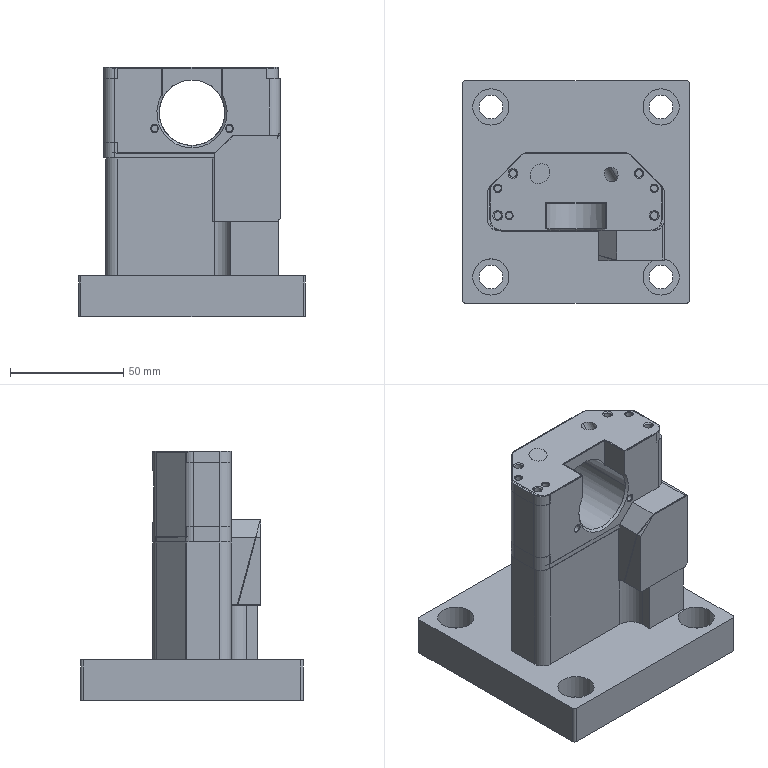NC program | NX | posted with a generic post | part box 100 x 98 x 110 mm
Lines 1874 to 3149 of 3149:
(FLOOR_WALL_2 , TOOL : D8-25-D8-60-3T-FINISH)
N3686 T27 M6
N3688 G54
N3690 G17 G43 G0 G90 X25.696 Y-29.571 B0. C219.917 S4500 H27 M3
N3692 Z33.
N3694 Z3.
N3696 G94 G1 Z0. F800.
N3698 X25.851 Y-29.385
N3700 G3 X25.601 Y-26.568 R2.
N3702 G1 X6.074 Y-10.231
N3704 X5.457 Y-3.296
N3706 X5.618 Y-3.103
N3708 X32.769 Y-25.818
N3710 X36.09 Y-21.849
N3712 X8.939 Y0.866
N3714 X12.259 Y4.835
N3716 X39.41 Y-17.88
N3718 X42.731 Y-13.911
N3720 X15.58 Y8.804
N3722 G3 X12.763 Y8.553 R2.
N3724 G1 X11.996 Y9.195
N3726 Z3.
N3728 G0 Z33.
(PLANAR_MILL_24_COPY , TOOL : D8-25-D8-60-3T-FINISH)
N3730 X12.191 Y-35.298
N3732 Z2.
N3734 Z-25.
N3736 G1 Z-28.
N3738 X6.055 Y-30.164
N3740 X-30.76 Y0.636
N3742 X-36.896 Y5.769
N3744 Z-25.
N3746 G0 Z2.
(FLOOR_WALL_1_COPY_2 , TOOL : D8-25-D8-60-3T-FINISH)
N3748 Z30.2
N3750 X18.538 Y-33.722
N3752 Z-27.
N3754 G1 Z-30.
N3756 X18.694 Y-33.536
N3758 G3 X18.443 Y-30.718 R2.
N3760 G1 X14.105 Y-27.089
N3762 X14.538 Y-26.57
N3764 X-28.719 Y9.62
N3766 X-29.153 Y9.102
N3768 X-33.492 Y12.732
N3770 X-34.28 Y21.599
N3772 X-34.289 Y21.703
N3774 X5.708 Y-11.76
N3776 X4.94 Y-3.134
N3778 X5.098 Y-2.945
N3780 X-31.333 Y27.534
N3782 X-27.247 Y32.419
N3784 X9.185 Y1.939
N3786 X13.271 Y6.824
N3788 X-23.06 Y37.22
N3790 G3 X-25.877 Y36.97 R2.
N3792 G1 X-26.744 Y37.695
N3794 Z-27.
N3796 G0 Z30.2
N3798 X24.693 Y-33.174
N3800 Z-27.
N3802 G1 Z-30.
N3804 X24.161 Y-27.198
N3806 X27.414 Y-29.92
N3808 G2 X27.665 Y-32.737 R2.
N3810 G1 X27.509 Y-32.924
N3812 Z-27.
N3814 G0 Z30.2
(PLANAR_MILL_25 , TOOL : D8-25-D8-60-3T-FINISH)
N3816 X38.714 Y-25.703
N3818 Z30.
N3820 Z-12.
N3822 G1 Z-15.
N3824 X30.745 Y-26.412
N3826 X18.702 Y-27.483
N3828 G2 X15.78 Y-26.566 R4.
N3830 G1 X7.809 Y-19.897
N3832 G2 X6.391 Y-17.184 R4.
N3834 G1 X5.294 Y-4.849
N3836 G2 X6.21 Y-1.928 R4.
N3838 G1 X22.564 Y17.619
N3840 X27.697 Y23.755
N3842 Z-12.
N3844 G0 Z30.
N3846 X38.714 Y-25.703
N3848 Z-12.
N3850 G1 Z-15.
N3852 X30.745 Y-26.412
N3854 X18.702 Y-27.483
N3856 G2 X15.78 Y-26.566 R4.
N3858 G1 X7.809 Y-19.897
N3860 G2 X6.391 Y-17.184 R4.
N3862 G1 X5.294 Y-4.849
N3864 G2 X6.21 Y-1.928 R4.
N3866 G1 X22.564 Y17.619
N3868 X27.697 Y23.755
N3870 Z-12.
N3872 G0 Z30.
N3874 X38.714 Y-25.703
N3876 Z-27.
N3878 G1 Z-30.
N3880 X30.745 Y-26.412
N3882 X18.702 Y-27.483
N3884 G2 X15.78 Y-26.566 R4.
N3886 G1 X7.809 Y-19.897
N3888 G2 X6.391 Y-17.184 R4.
N3890 G1 X5.294 Y-4.849
N3892 G2 X6.21 Y-1.928 R4.
N3894 G1 X22.564 Y17.619
N3896 X27.697 Y23.755
N3898 Z-27.
N3900 G0 Z30.
N3902 X38.714 Y-25.703
N3904 Z-27.
N3906 G1 Z-30.
N3908 X30.745 Y-26.412
N3910 X18.702 Y-27.483
N3912 G2 X15.78 Y-26.566 R4.
N3914 G1 X7.809 Y-19.897
N3916 G2 X6.391 Y-17.184 R4.
N3918 G1 X5.294 Y-4.849
N3920 G2 X6.21 Y-1.928 R4.
N3922 G1 X22.564 Y17.619
N3924 X27.697 Y23.755
N3926 Z-27.
N3928 G0 Z30.
(PLANAR_MILL_25_COPY_2 , TOOL : D8-25-D8-60-3T-FINISH)
N3930 X1.13 Y-8.108
N3932 Z-11.998
N3934 G1 Z-14.998
N3936 X6.264 Y-1.973
N3938 X22.617 Y17.574
N3940 X27.751 Y23.71
N3942 Z-11.998
N3944 G0 Z30.
N3946 X1.13 Y-8.108
N3948 Z-26.996
N3950 G1 Z-29.996
N3952 X6.264 Y-1.973
N3954 X22.617 Y17.574
N3956 X27.751 Y23.71
N3958 Z-26.996
N3960 G0 Z30.
(PLANAR_MILL_25_COPY_1 , TOOL : D8-25-D8-60-3T-FINISH)
N3962 X-37.05 Y-0.649
N3964 Z2.
N3966 Z-26.996
N3968 G1 Z-29.996
N3970 X-31.916 Y5.487
N3972 X-31.261 Y6.27
N3974 G2 X-25.626 Y6.772 R4.
N3976 G1 X11.189 Y-24.029
N3978 G2 X11.69 Y-29.663 R4.
N3980 G1 X11.034 Y-30.447
N3982 X5.901 Y-36.583
N3984 Z-26.996
N3986 G0 Z2.
N3988 X-37.05 Y-0.649
N3990 Z-26.996
N3992 G1 Z-29.996
N3994 X-31.916 Y5.487
N3996 X-31.261 Y6.27
N3998 G2 X-25.626 Y6.772 R4.
N4000 G1 X11.189 Y-24.029
N4002 G2 X11.69 Y-29.663 R4.
N4004 G1 X11.034 Y-30.447
N4006 X5.901 Y-36.583
N4008 Z-26.996
N4010 G0 Z2.
(FLOOR_WALL_1_COPY_3_COPY , TOOL : D8-25-D8-60-3T-FINISH)
N4012 Z30.
N4014 X0.916 Y-11.523
N4016 Z-26.1
N4018 G1 Z-29.1
N4020 X-1.009 Y-13.824
N4022 X-7.425 Y-21.494
N4024 X-11.566 Y-18.03
N4026 X-5.15 Y-10.36
N4028 X-9.29 Y-6.895
N4030 X-15.707 Y-14.565
N4032 X-19.848 Y-11.101
N4034 X-13.431 Y-3.431
N4036 X-11.506 Y-1.13
N4038 Z-26.1
N4040 G0 Z30.
(PLANAR_MILL_35_COPY , TOOL : D8-25-D8-60-3T-FINISH)
N4042 X-36.493 Y24.952
N4044 Z0.
N4046 Z-33.
N4048 G1 Z-35.
N4050 G3 X-33.675 Y25.202 R2.
N4052 G1 X-24.353 Y36.346
N4054 G2 X-11.675 Y37.474 R9.
N4056 G3 X-8.857 Y37.724 R2.
N4058 G1 Z-33.
N4060 G0 Z0.
(FLOOR_WALL_1_COPY_1_1_COPY , TOOL : D8-25-D8-60-3T-FINISH)
N4062 G3P2 X0. Y0. Z0. I0. J74.9748 K-39.9168
N4064 G53.1
N4066 X22.176 Y-36.663 Z55.558 H27
N4068 Z22.558
N4070 G1 Z19.558
N4072 X18.977 Y-39.339
N4074 X-4.808 Y-59.239
N4076 X-8.388 Y-54.96
N4078 X18.763 Y-32.245
N4080 X15.183 Y-27.966
N4082 X-11.968 Y-50.681
N4084 X-15.548 Y-46.402
N4086 X11.603 Y-23.686
N4088 X8.023 Y-19.407
N4090 X-19.128 Y-42.123
N4092 X-22.708 Y-37.844
N4094 X4.443 Y-15.128
N4096 X0.863 Y-10.849
N4098 X-26.288 Y-33.564
N4100 X-28.589 Y-35.489
N4102 Z22.558
N4104 G0 Z55.558
N4106 G69
N4108 M5
(DRILLING_7 , TOOL : 点孔D6-65-90度)
N4110 T04 M6
N4112 G54
N4114 G17 G43 G0 G90 X-2.363 Y-13.734 B0. C219.917 S2500 H4 M3
N4116 Z-27.
N4118 G94 G81 G98 Z-32. F200. R-27.
N4120 X-13.101 Y-4.75
N4122 X-16.573 Y20.71
N4124 G80
N4126 M5
(DRILLING_1_COPY , TOOL : D6-18-D6-50-3T-ROUGH)
N4128 T33 M6
N4130 G54
N4132 G17 G0 G90 X21.776 Y-11.374 B0. C219.917 S1600 M3
N4134 G43 Z3. H33
N4136 G94 G83 G99 Z-22.6 F150. Q5. R3.
N4138 G80
N4140 M5
(SPOT_DRILLING_14 , TOOL : 钻头D3.3-45-73)
N4142 T10 M6
N4144 G54
N4146 G17 G0 G90 X-2.363 Y-13.734 B0. C219.917 S3000 M3
N4148 G43 Z0. H10
N4150 G94 G81 G98 Z-39. F200. R-27.
N4152 X-13.101 Y-4.75
N4154 G80
N4156 M5
(DRILLING_9 , TOOL : D15.3)
N4158 T29 M6
N4160 G54
N4162 G17 G0 G90 X-16.573 Y20.71 B0. C219.917 S1600 M3
N4164 G43 Z-27. H29
N4166 G94 G83 G99 Z-56.797 F150. Q5. R-27.
N4168 G80
N4170 M5
(PLANAR_MILL_37 , TOOL : D8-25-D8-60-3T-ROUGH)
N4172 T26 M6
N4174 G54
N4176 G17 G0 G90 X19.98 Y-10.783 B0. C219.917 S4500 M3
N4178 G43 Z30. H26
N4180 Z2.
N4182 G94 G1 X19.859 Y-11.154 Z1.98 F1000.
N4184 X19.928 Y-11.929 Z1.939
N4186 X20.297 Y-12.613 Z1.898
N4188 X20.817 Y-13.048 Z1.863
N4190 X21.556 Y-13.291 Z1.822
N4192 X22.331 Y-13.222 Z1.781
N4194 X23.016 Y-12.853 Z1.74
N4196 X23.451 Y-12.333 Z1.705
N4198 X23.694 Y-11.594 Z1.664
N4200 X23.625 Y-10.819 Z1.623
N4202 X23.255 Y-10.134 Z1.582
N4204 X22.735 Y-9.699 Z1.547
N4206 X21.996 Y-9.456 Z1.506
N4208 X21.221 Y-9.525 Z1.465
N4210 X20.536 Y-9.894 Z1.424
N4212 X20.101 Y-10.414 Z1.389
N4214 X19.859 Y-11.154 Z1.348
N4216 X19.928 Y-11.929 Z1.307
N4218 X20.297 Y-12.613 Z1.267
N4220 X20.817 Y-13.048 Z1.231
N4222 X21.556 Y-13.291 Z1.19
N4224 X22.331 Y-13.222 Z1.15
N4226 X23.016 Y-12.853 Z1.109
N4228 X23.451 Y-12.333 Z1.073
N4230 X23.694 Y-11.594 Z1.032
N4232 X23.625 Y-10.819 Z0.992
N4234 X23.255 Y-10.134 Z0.951
N4236 X22.735 Y-9.699 Z0.915
N4238 X21.996 Y-9.456 Z0.875
N4240 X21.221 Y-9.525 Z0.834
N4242 X20.536 Y-9.894 Z0.793
N4244 X20.101 Y-10.414 Z0.758
N4246 X19.859 Y-11.154 Z0.717
N4248 X19.928 Y-11.929 Z0.676
N4250 X20.297 Y-12.613 Z0.635
N4252 X20.817 Y-13.048 Z0.6
N4254 X21.556 Y-13.291 Z0.559
N4256 X22.331 Y-13.222 Z0.518
N4258 X23.016 Y-12.853 Z0.477
N4260 X23.451 Y-12.333 Z0.442
N4262 X23.694 Y-11.594 Z0.401
N4264 X23.625 Y-10.819 Z0.36
N4266 X23.255 Y-10.134 Z0.32
N4268 X22.735 Y-9.699 Z0.284
N4270 X21.996 Y-9.456 Z0.243
N4272 X21.221 Y-9.525 Z0.202
N4274 X20.536 Y-9.894 Z0.162
N4276 X20.101 Y-10.414 Z0.126
N4278 X19.859 Y-11.154 Z0.085
N4280 X19.928 Y-11.929 Z0.045
N4282 X20.297 Y-12.613 Z0.004
N4284 X20.817 Y-13.048 Z-0.032
N4286 X21.556 Y-13.291 Z-0.073
N4288 X22.331 Y-13.222 Z-0.113
N4290 X23.016 Y-12.853 Z-0.154
N4292 X23.451 Y-12.333 Z-0.19
N4294 X23.694 Y-11.594 Z-0.23
N4296 X23.625 Y-10.819 Z-0.271
N4298 X23.255 Y-10.134 Z-0.312
N4300 X22.735 Y-9.699 Z-0.347
N4302 X21.996 Y-9.456 Z-0.388
N4304 X21.221 Y-9.525 Z-0.429
N4306 X20.536 Y-9.894 Z-0.47
N4308 X20.101 Y-10.414 Z-0.505
N4310 X19.859 Y-11.154 Z-0.546
N4312 X19.928 Y-11.929 Z-0.587
N4314 X20.297 Y-12.613 Z-0.628
N4316 X20.817 Y-13.048 Z-0.663
N4318 X21.556 Y-13.291 Z-0.704
N4320 X22.331 Y-13.222 Z-0.745
N4322 X23.016 Y-12.853 Z-0.785
N4324 X23.451 Y-12.333 Z-0.821
N4326 X23.694 Y-11.594 Z-0.862
N4328 X23.625 Y-10.819 Z-0.903
N4330 X23.255 Y-10.134 Z-0.943
N4332 X22.735 Y-9.699 Z-0.979
N4334 X21.996 Y-9.456 Z-1.02
N4336 X21.221 Y-9.525 Z-1.06
N4338 X20.536 Y-9.894 Z-1.101
N4340 X20.101 Y-10.414 Z-1.137
N4342 X19.859 Y-11.154 Z-1.177
N4344 X19.928 Y-11.929 Z-1.218
N4346 X20.297 Y-12.613 Z-1.259
N4348 X20.817 Y-13.048 Z-1.295
N4350 X21.556 Y-13.291 Z-1.335
N4352 X22.331 Y-13.222 Z-1.376
N4354 X23.016 Y-12.853 Z-1.417
N4356 X23.451 Y-12.333 Z-1.452
N4358 X23.694 Y-11.594 Z-1.493
N4360 X23.625 Y-10.819 Z-1.534
N4362 X23.255 Y-10.134 Z-1.575
N4364 X22.735 Y-9.699 Z-1.61
N4366 X21.996 Y-9.456 Z-1.651
N4368 X21.221 Y-9.525 Z-1.692
N4370 X20.536 Y-9.894 Z-1.733
N4372 X20.101 Y-10.414 Z-1.768
N4374 X19.859 Y-11.154 Z-1.809
N4376 X19.928 Y-11.929 Z-1.85
N4378 X20.297 Y-12.613 Z-1.89
N4380 X20.817 Y-13.048 Z-1.926
N4382 X21.556 Y-13.291 Z-1.967
N4384 X22.331 Y-13.222 Z-2.008
N4386 X23.016 Y-12.853 Z-2.048
N4388 X23.451 Y-12.333 Z-2.084
N4390 X23.694 Y-11.594 Z-2.125
N4392 X23.625 Y-10.819 Z-2.165
N4394 X23.255 Y-10.134 Z-2.206
N4396 X22.735 Y-9.699 Z-2.242
N4398 X21.996 Y-9.456 Z-2.282
N4400 X21.221 Y-9.525 Z-2.323
N4402 X20.536 Y-9.894 Z-2.364
N4404 X20.101 Y-10.414 Z-2.4
N4406 X19.859 Y-11.154 Z-2.44
N4408 X19.928 Y-11.929 Z-2.481
N4410 X20.297 Y-12.613 Z-2.522
N4412 X20.817 Y-13.048 Z-2.557
N4414 X21.556 Y-13.291 Z-2.598
N4416 X22.331 Y-13.222 Z-2.639
N4418 X23.016 Y-12.853 Z-2.68
N4420 X23.451 Y-12.333 Z-2.715
N4422 X23.694 Y-11.594 Z-2.756
N4424 X23.625 Y-10.819 Z-2.797
N4426 X23.255 Y-10.134 Z-2.838
N4428 X22.735 Y-9.699 Z-2.873
N4430 X21.996 Y-9.456 Z-2.914
N4432 X21.221 Y-9.525 Z-2.955
N4434 X20.536 Y-9.894 Z-2.995
N4436 X20.101 Y-10.414 Z-3.031
N4438 X19.859 Y-11.154 Z-3.072
N4440 X19.928 Y-11.929 Z-3.112
N4442 X20.297 Y-12.613 Z-3.153
N4444 X20.817 Y-13.048 Z-3.189
N4446 X21.556 Y-13.291 Z-3.23
N4448 X22.331 Y-13.222 Z-3.27
N4450 X23.016 Y-12.853 Z-3.311
N4452 X23.451 Y-12.333 Z-3.347
N4454 X23.694 Y-11.594 Z-3.387
N4456 X23.625 Y-10.819 Z-3.428
N4458 X23.255 Y-10.134 Z-3.469
N4460 X22.735 Y-9.699 Z-3.504
N4462 X21.996 Y-9.456 Z-3.545
N4464 X21.221 Y-9.525 Z-3.586
N4466 X20.536 Y-9.894 Z-3.627
N4468 X20.101 Y-10.414 Z-3.662
N4470 X19.859 Y-11.154 Z-3.703
N4472 X19.928 Y-11.929 Z-3.744
N4474 X20.297 Y-12.613 Z-3.785
N4476 X20.817 Y-13.048 Z-3.82
N4478 X21.556 Y-13.291 Z-3.861
N4480 X22.331 Y-13.222 Z-3.902
N4482 X23.016 Y-12.853 Z-3.943
N4484 X23.451 Y-12.333 Z-3.978
N4486 X23.694 Y-11.594 Z-4.019
N4488 X23.625 Y-10.819 Z-4.06
N4490 X23.255 Y-10.134 Z-4.1
N4492 X22.735 Y-9.699 Z-4.136
N4494 X21.996 Y-9.456 Z-4.177
N4496 X21.221 Y-9.525 Z-4.217
N4498 X20.536 Y-9.894 Z-4.258
N4500 X20.101 Y-10.414 Z-4.294
N4502 X19.859 Y-11.154 Z-4.335
N4504 X19.928 Y-11.929 Z-4.375
N4506 X20.297 Y-12.613 Z-4.416
N4508 X20.817 Y-13.048 Z-4.452
N4510 X21.556 Y-13.291 Z-4.492
N4512 X22.331 Y-13.222 Z-4.533
N4514 X23.016 Y-12.853 Z-4.574
N4516 X23.451 Y-12.333 Z-4.609
N4518 X23.694 Y-11.594 Z-4.65
N4520 X23.625 Y-10.819 Z-4.691
N4522 X23.255 Y-10.134 Z-4.732
N4524 X22.735 Y-9.699 Z-4.767
N4526 X21.996 Y-9.456 Z-4.808
N4528 X21.221 Y-9.525 Z-4.849
N4530 X20.536 Y-9.894 Z-4.89
N4532 X20.101 Y-10.414 Z-4.925
N4534 X19.859 Y-11.154 Z-4.966
N4536 X19.928 Y-11.929 Z-5.007
N4538 X20.297 Y-12.613 Z-5.047
N4540 X20.817 Y-13.048 Z-5.083
N4542 X21.556 Y-13.291 Z-5.124
N4544 X22.331 Y-13.222 Z-5.165
N4546 X23.016 Y-12.853 Z-5.205
N4548 X23.451 Y-12.333 Z-5.241
N4550 X23.694 Y-11.594 Z-5.282
N4552 X23.625 Y-10.819 Z-5.322
N4554 X23.255 Y-10.134 Z-5.363
N4556 X22.735 Y-9.699 Z-5.399
N4558 X21.996 Y-9.456 Z-5.439
N4560 X21.221 Y-9.525 Z-5.48
N4562 X20.536 Y-9.894 Z-5.521
N4564 X20.101 Y-10.414 Z-5.557
N4566 X19.859 Y-11.154 Z-5.597
N4568 X19.928 Y-11.929 Z-5.638
N4570 X20.297 Y-12.613 Z-5.679
N4572 X20.817 Y-13.048 Z-5.714
N4574 X21.556 Y-13.291 Z-5.755
N4576 X22.331 Y-13.222 Z-5.796
N4578 X23.016 Y-12.853 Z-5.837
N4580 X23.451 Y-12.333 Z-5.872
N4582 X23.694 Y-11.594 Z-5.913
N4584 X23.625 Y-10.819 Z-5.954
N4586 X23.255 Y-10.134 Z-5.995
N4588 X22.735 Y-9.699 Z-6.03
N4590 X21.996 Y-9.456 Z-6.071
N4592 X21.221 Y-9.525 Z-6.112
N4594 X20.536 Y-9.894 Z-6.152
N4596 X20.101 Y-10.414 Z-6.188
N4598 X19.859 Y-11.154 Z-6.229
N4600 X19.928 Y-11.929 Z-6.27
N4602 X20.297 Y-12.613 Z-6.31
N4604 X20.817 Y-13.048 Z-6.346
N4606 X21.556 Y-13.291 Z-6.387
N4608 X22.331 Y-13.222 Z-6.427
N4610 X23.016 Y-12.853 Z-6.468
N4612 X23.451 Y-12.333 Z-6.504
N4614 X23.694 Y-11.594 Z-6.544
N4616 X23.625 Y-10.819 Z-6.585
N4618 X23.255 Y-10.134 Z-6.626
N4620 X22.735 Y-9.699 Z-6.662
N4622 X21.996 Y-9.456 Z-6.702
N4624 X21.221 Y-9.525 Z-6.743
N4626 X20.536 Y-9.894 Z-6.784
N4628 X20.101 Y-10.414 Z-6.819
N4630 X19.859 Y-11.154 Z-6.86
N4632 X19.928 Y-11.929 Z-6.901
N4634 X20.297 Y-12.613 Z-6.942
N4636 X20.817 Y-13.048 Z-6.977
N4638 X21.556 Y-13.291 Z-7.018
N4640 X22.331 Y-13.222 Z-7.059
N4642 X23.016 Y-12.853 Z-7.1
N4644 X23.451 Y-12.333 Z-7.135
N4646 X23.694 Y-11.594 Z-7.176
N4648 X23.625 Y-10.819 Z-7.217
N4650 X23.255 Y-10.134 Z-7.257
N4652 X22.735 Y-9.699 Z-7.293
N4654 X21.996 Y-9.456 Z-7.334
N4656 X21.221 Y-9.525 Z-7.374
N4658 X20.536 Y-9.894 Z-7.415
N4660 X20.101 Y-10.414 Z-7.451
N4662 X19.859 Y-11.154 Z-7.492
N4664 X19.928 Y-11.929 Z-7.532
N4666 X20.297 Y-12.613 Z-7.573
N4668 X20.817 Y-13.048 Z-7.609
N4670 X21.556 Y-13.291 Z-7.649
N4672 X22.331 Y-13.222 Z-7.69
N4674 X23.016 Y-12.853 Z-7.731
N4676 X23.451 Y-12.333 Z-7.766
N4678 X23.694 Y-11.594 Z-7.807
N4680 X23.625 Y-10.819 Z-7.848
N4682 X23.255 Y-10.134 Z-7.889
N4684 X22.735 Y-9.699 Z-7.924
N4686 X21.996 Y-9.456 Z-7.965
N4688 X21.221 Y-9.525 Z-8.006
N4690 X20.536 Y-9.894 Z-8.047
N4692 X20.101 Y-10.414 Z-8.082
N4694 X19.859 Y-11.154 Z-8.123
N4696 X19.928 Y-11.929 Z-8.164
N4698 X20.297 Y-12.613 Z-8.205
N4700 X20.817 Y-13.048 Z-8.24
N4702 X21.556 Y-13.291 Z-8.281
N4704 X22.331 Y-13.222 Z-8.322
N4706 X23.016 Y-12.853 Z-8.362
N4708 X23.451 Y-12.333 Z-8.398
N4710 X23.694 Y-11.594 Z-8.439
N4712 X23.625 Y-10.819 Z-8.479
N4714 X23.255 Y-10.134 Z-8.52
N4716 X22.735 Y-9.699 Z-8.556
N4718 X21.996 Y-9.456 Z-8.597
N4720 X21.221 Y-9.525 Z-8.637
N4722 X20.536 Y-9.894 Z-8.678
N4724 X20.101 Y-10.414 Z-8.714
N4726 X19.859 Y-11.154 Z-8.754
N4728 X19.928 Y-11.929 Z-8.795
N4730 X20.297 Y-12.613 Z-8.836
N4732 X20.817 Y-13.048 Z-8.871
N4734 X21.556 Y-13.291 Z-8.912
N4736 X22.331 Y-13.222 Z-8.953
N4738 X23.016 Y-12.853 Z-8.994
N4740 X23.451 Y-12.333 Z-9.029
N4742 X23.694 Y-11.594 Z-9.07
N4744 X23.625 Y-10.819 Z-9.111
N4746 X23.255 Y-10.134 Z-9.152
N4748 X22.735 Y-9.699 Z-9.187
N4750 X21.996 Y-9.456 Z-9.228
N4752 X21.221 Y-9.525 Z-9.269
N4754 X20.536 Y-9.894 Z-9.309
N4756 X20.101 Y-10.414 Z-9.345
N4758 X19.859 Y-11.154 Z-9.386
N4760 X19.928 Y-11.929 Z-9.427
N4762 X20.297 Y-12.613 Z-9.467
N4764 X20.817 Y-13.048 Z-9.503
N4766 X21.556 Y-13.291 Z-9.544
N4768 X22.331 Y-13.222 Z-9.584
N4770 X23.016 Y-12.853 Z-9.625
N4772 X23.451 Y-12.333 Z-9.661
N4774 X23.694 Y-11.594 Z-9.701
N4776 X23.625 Y-10.819 Z-9.742
N4778 X23.255 Y-10.134 Z-9.783
N4780 X22.735 Y-9.699 Z-9.819
N4782 X21.996 Y-9.456 Z-9.859
N4784 X21.221 Y-9.525 Z-9.9
N4786 X20.536 Y-9.894 Z-9.941
N4788 X20.101 Y-10.414 Z-9.976
N4790 X19.859 Y-11.154 Z-10.017
N4792 X19.928 Y-11.929 Z-10.058
N4794 X20.297 Y-12.613 Z-10.099
N4796 X20.817 Y-13.048 Z-10.134
N4798 X21.556 Y-13.291 Z-10.175
N4800 X22.331 Y-13.222 Z-10.216
N4802 X23.016 Y-12.853 Z-10.257
N4804 X23.451 Y-12.333 Z-10.292
N4806 X23.694 Y-11.594 Z-10.333
N4808 X23.625 Y-10.819 Z-10.374
N4810 X23.255 Y-10.134 Z-10.414
N4812 X22.735 Y-9.699 Z-10.45
N4814 X21.996 Y-9.456 Z-10.491
N4816 X21.221 Y-9.525 Z-10.532
N4818 X20.536 Y-9.894 Z-10.572
N4820 X20.101 Y-10.414 Z-10.608
N4822 X19.859 Y-11.154 Z-10.649
N4824 X19.928 Y-11.929 Z-10.689
N4826 X20.297 Y-12.613 Z-10.73
N4828 X20.817 Y-13.048 Z-10.766
N4830 X21.556 Y-13.291 Z-10.806
N4832 X22.331 Y-13.222 Z-10.847
N4834 X23.016 Y-12.853 Z-10.888
N4836 X23.451 Y-12.333 Z-10.924
N4838 X23.694 Y-11.594 Z-10.964
N4840 X23.625 Y-10.819 Z-11.005
N4842 X23.255 Y-10.134 Z-11.046
N4844 X22.735 Y-9.699 Z-11.081
N4846 X21.996 Y-9.456 Z-11.122
N4848 X21.221 Y-9.525 Z-11.163
N4850 X20.536 Y-9.894 Z-11.204
N4852 X20.101 Y-10.414 Z-11.239
N4854 X19.859 Y-11.154 Z-11.28
N4856 X19.928 Y-11.929 Z-11.321
N4858 X20.297 Y-12.613 Z-11.362
N4860 X20.817 Y-13.048 Z-11.397
N4862 X21.556 Y-13.291 Z-11.438
N4864 X22.331 Y-13.222 Z-11.479
N4866 X23.016 Y-12.853 Z-11.519
N4868 X23.451 Y-12.333 Z-11.555
N4870 X23.694 Y-11.594 Z-11.596
N4872 X23.625 Y-10.819 Z-11.636
N4874 X23.255 Y-10.134 Z-11.677
N4876 X22.735 Y-9.699 Z-11.713
N4878 X21.996 Y-9.456 Z-11.754
N4880 X21.221 Y-9.525 Z-11.794
N4882 X20.536 Y-9.894 Z-11.835
N4884 X20.101 Y-10.414 Z-11.871
N4886 X19.859 Y-11.154 Z-11.911
N4888 X19.928 Y-11.929 Z-11.952
N4890 X20.297 Y-12.613 Z-11.993
N4892 X20.817 Y-13.048 Z-12.029
N4894 X21.556 Y-13.291 Z-12.069
N4896 X22.331 Y-13.222 Z-12.11
N4898 X23.016 Y-12.853 Z-12.151
N4900 X23.451 Y-12.333 Z-12.186
N4902 X23.694 Y-11.594 Z-12.227
N4904 X23.625 Y-10.819 Z-12.268
N4906 X23.255 Y-10.134 Z-12.309
N4908 X22.735 Y-9.699 Z-12.344
N4910 X21.996 Y-9.456 Z-12.385
N4912 X21.221 Y-9.525 Z-12.426
N4914 X20.536 Y-9.894 Z-12.467
N4916 X20.101 Y-10.414 Z-12.502
N4918 X19.859 Y-11.154 Z-12.543
N4920 X19.928 Y-11.929 Z-12.584
N4922 X20.297 Y-12.613 Z-12.624
N4924 X20.817 Y-13.048 Z-12.66
N4926 X21.556 Y-13.291 Z-12.701
N4928 X22.331 Y-13.222 Z-12.741
N4930 X23.016 Y-12.853 Z-12.782
N4932 X23.234 Y-12.593 Z-12.8
N4934 G3 X22.995 Y-9.916 R1.9
N4936 X23.234 Y-12.593 R-1.9
N4938 G1 Z-10.8
N4940 G0 Z30.
N4942 M5
(PLANAR_MILL_26_COPY_1 , TOOL : T-2)
N4944 T30 M6
N4946 G54
N4948 G17 G0 G90 X22.146 Y-12.248 B0. C219.917 S3000 M3
N4950 G43 Z20. H30
N4952 Z-10.9
N4954 G94 G1 Z-12.9 F500.
N4956 X22.63 Y-13.392
N4958 G3 X24.039 Y-13.266 R1.
N4960 X23.669 Y-9.111 R2.95
N4962 X24.039 Y-13.266 R-2.95
N4964 X23.914 Y-11.858 R1.
N4966 G1 X22.703 Y-11.583
N4968 Z-10.9
N4970 G0 Z20.
(PLANAR_MILL_26_COPY_COPY , TOOL : T-2)
N4972 X21.776 Y-11.374
N4974 Z-9.5
N4976 G1 Z-11.5
N4978 X21.225 Y-9.793
N4980 G3 X19.514 Y-9.481 R1.
N4982 X19.883 Y-13.636 R2.95
N4984 X19.514 Y-9.481 R-2.95
N4986 X20.123 Y-11.11 R1.
N4988 G1 X21.776 Y-11.374
N4990 Z-9.5
N4992 G0 Z20.
(PLANAR_MILL_26 , TOOL : T-2)
N4994 X21.797 Y-11.419
N4996 Z-11.
N4998 G1 Z-13.
N5000 X22.707 Y-13.456
N5002 G3 X24.116 Y-13.331 R1.
N5004 X23.733 Y-9.034 R3.05
N5006 X24.116 Y-13.331 R-3.05
N5008 X23.99 Y-11.922 R1.
N5010 G1 X21.825 Y-11.386
N5012 Z-11.
N5014 G0 Z20.
(PLANAR_MILL_26_COPY , TOOL : T-2)
N5016 X21.797 Y-11.419
N5018 Z-9.5
N5020 G1 Z-11.5
N5022 X22.707 Y-13.456
N5024 G3 X24.116 Y-13.331 R1.
N5026 X23.733 Y-9.034 R3.05
N5028 X24.116 Y-13.331 R-3.05
N5030 X23.99 Y-11.922 R1.
N5032 G1 X21.825 Y-11.386
N5034 Z-9.5
N5036 G0 Z20.
N5038 M5
(PLANAR_MILL_27 , TOOL : 点孔D8-79-90度)
N5040 T15 M6
N5042 G54
N5044 G17 G0 G90 X44.349 Y-5.603 B0. C219.917 S3500 M3
N5046 G43 Z30. H15
N5048 Z0.
N5050 G94 G1 Z-2. F1000.
N5052 X43.065 Y-7.137
N5054 G2 X43.781 Y-8.619 R2.
N5056 G1 X43.789 Y-8.906
N5058 G2 X43.323 Y-10.242 R2.
N5060 G1 X32.247 Y-23.481
N5062 G2 X30.89 Y-24.19 R2.
N5064 G1 X18.589 Y-25.284
N5066 G2 X17.129 Y-24.826 R2.
N5068 G1 X9.284 Y-18.263
N5070 G2 X8.575 Y-16.906 R2.
N5072 G1 X7.493 Y-4.736
N5074 G2 X7.951 Y-3.276 R2.
N5076 G1 X19.087 Y10.035
N5078 G2 X20.319 Y10.729 R2.
N5080 G1 X20.604 Y10.772
N5082 G2 X22.189 Y10.329 R2.
N5084 G1 X43.065 Y-7.137
N5086 X44.349 Y-5.603
N5088 Z0.
N5090 G0 Z30.
(PLANAR_MILL_27_COPY , TOOL : 点孔D8-79-90度)
N5092 X21.656 Y-9.477
N5094 Z-1.
N5096 G1 Z-3.
N5098 X21.602 Y-8.62
N5100 G3 X18.785 Y-8.871 R2.
N5102 X19.274 Y-14.365 R3.9
N5104 X18.785 Y-8.871 R-3.9
N5106 X19.036 Y-11.688 R2.
N5108 G1 X19.889 Y-11.59
N5110 Z-1.
N5112 G0 Z30.
(PLANAR_MILL_27_COPY_COPY , TOOL : 点孔D8-79-90度)
N5114 X-18.056 Y24.559
N5116 Z0.
N5118 Z-30.5
N5120 G1 Z-32.5
N5122 X-18.453 Y24.891
N5124 G3 X-21.27 Y24.64 R2.
N5126 X-20.503 Y16.012 R6.125
N5128 X-21.27 Y24.64 R-6.125
N5130 X-21.02 Y21.823 R2.
N5132 G1 X-20.623 Y21.491
N5134 Z-30.5
N5136 G0 Z0.
(PLANAR_MILL_28 , TOOL : 点孔D8-79-90度)
N5138 Z10.
N5140 X-34.368 Y4.524
N5142 Z-31.5
N5144 G1 Z-33.5
N5146 G3 X-32.553 Y6.694 R2.
N5148 G1 X-33.882 Y21.635
N5150 G2 X-33.908 Y22.697 R8.3
N5152 X-33.095 Y24.805 R3.5
N5154 G1 X-23.816 Y35.897
N5156 G2 X-12.124 Y36.937 R8.3
N5158 G1 X15.487 Y13.836
N5160 G3 X18.305 Y14.087 R2.
N5162 G1 Z-31.5
N5164 G0 Z10.
N5166 X30.841 Y-30.834
N5168 Z-31.5
N5170 G1 Z-33.5
N5172 G3 X28.437 Y-29.344 R2.
N5174 G2 X27.275 Y-29.531 R8.3
N5176 G1 X12.334 Y-30.86
N5178 G3 X10.519 Y-33.03 R2.
N5180 G1 Z-31.5
N5182 G0 Z10.
(PLANAR_MILL_28_COPY_1 , TOOL : 点孔D8-79-90度)
N5184 X-34.874 Y27.509
N5186 Z-36.5
N5188 G1 Z-38.5
N5190 G3 X-32.057 Y27.76 R2.
N5192 G1 X-24.659 Y36.602
N5194 G3 X-24.91 Y39.42 R2.
N5196 G1 Z-36.5
N5198 G0 Z10.
(PLANAR_MILL_28_COPY , TOOL : 点孔D8-79-90度)
N5200 X-18.889 Y-1.929
N5202 Z2.
N5204 Z-26.8
N5206 G1 Z-28.8
N5208 G3 X-18.764 Y-3.337 R1.
N5210 G2 X-18.664 Y-4.464 R0.8
N5212 G1 X-19.755 Y-5.768
N5214 G2 X-20.881 Y-5.868 R0.8
N5216 G1 X-27.615 Y-0.235
N5218 G2 X-29.459 Y2.682 R5.65
N5220 X-29.298 Y3.396 R0.8
N5222 G1 X-28.788 Y4.006
N5224 G2 X-27.661 Y4.106 R0.8
N5226 G1 X-18.764 Y-3.337
N5228 G3 X-17.355 Y-3.212 R1.
N5230 G1 Z-26.8
N5232 G0 Z2.
N5234 X9.923 Y-28.113
N5236 Z-26.8
N5238 G1 Z-28.8
N5240 G3 X8.514 Y-28.239 R1.
N5242 G2 X7.84 Y-28.523 R0.8
N5244 X4.643 Y-27.223 R5.65
N5246 G1 X-2.09 Y-21.589
N5248 G2 X-2.191 Y-20.462 R0.8
N5250 G1 X-1.1 Y-19.159
N5252 G2 X0.027 Y-19.058 R0.8
N5254 G1 X8.924 Y-26.502
N5256 G2 X9.024 Y-27.629 R0.8
N5258 G1 X8.514 Y-28.239
N5260 G3 X8.639 Y-29.647 R1.
N5262 G1 Z-26.8
N5264 G0 Z2.
(PLANAR_MILL_28_COPY_COPY , TOOL : 点孔D8-79-90度)
N5266 X-15.553 Y-4.72
N5268 Z0.9
N5270 Z-27.9
N5272 G1 Z-29.9
N5274 G3 X-15.428 Y-6.129 R1.
N5276 G1 X-3.309 Y-16.267
N5278 G3 X-1.901 Y-16.142 R1.
N5280 G1 Z-27.9
N5282 G0 Z0.9
N5284 X-5.302 Y-20.207
N5286 Z-27.9
N5288 G1 Z-29.9
N5290 G3 X-5.427 Y-18.798 R1.
N5292 G1 X-17.545 Y-8.66
N5294 G3 X-18.954 Y-8.785 R1.
N5296 G1 Z-27.9
N5298 G0 Z0.9
(PLANAR_MILL_9_COPY_COPY_COPY , TOOL : 点孔D8-79-90度)
N5300 G3P2 X0. Y0. Z0. I0. J74.9748 K-39.9168
N5302 G53.1
N5304 X2.605 Y-43.689 Z49.558 H15
N5306 Z19.058
N5308 G1 Z17.058
N5310 X2.814 Y-43.939
N5312 G3 X5.632 Y-44.19 R2.
N5314 X6.672 Y-32.498 R8.3
N5316 X5.632 Y-44.19 R-8.3
N5318 X5.882 Y-41.372 R2.
N5320 G1 X5.673 Y-41.122
N5322 Z19.058
N5324 G0 Z49.558
(PLANAR_MILL_9_COPY_COPY , TOOL : 点孔D8-79-90度)
N5326 X0.605 Y-62.748
N5328 Z19.558
N5330 G1 Z17.558
N5332 X-1.962 Y-59.68
N5334 X-27.009 Y-29.742
N5336 X-29.576 Y-26.674
N5338 Z19.558
N5340 G0 Z49.558
(PLANAR_MILL_9_COPY_COPY_COPY_1 , TOOL : 点孔D8-79-90度)
N5342 X-5.416 Y-6.461
N5344 Z19.558
N5346 G1 Z17.558
N5348 X-2.85 Y-9.529
N5350 X16.813 Y-33.031
N5352 G2 X17.274 Y-34.457 R2.
N5354 G1 X16.465 Y-45.779
N5356 X16.18 Y-49.769
N5358 Z19.558
N5360 G0 Z49.558
(PLANAR_MILL_9_COPY_COPY_COPY_1_COPY , TOOL : 点孔D8-79-90度)
N5362 X18.983 Y-44.508
N5364 Z19.558
N5366 G1 Z17.558
N5368 X15.915 Y-47.074
N5370 X0.583 Y-59.901
N5372 X-2.485 Y-62.468
N5374 Z19.558
N5376 G0 Z49.558
N5378 G69
N5380 M5
(THREAD_MILLING_2_1 , TOOL : G1-2)
N5382 T18 M6
N5384 G54
N5386 G3P2 X0. Y0. Z0. I0. J74.9748 K-39.9168
N5388 G53.1
N5390 G17 G43 G0 G90 X0.306 Y-37.824 Z49.558 S4500 H18 M3
N5392 Z-0.63
N5394 G41 G94 G1 X-1.059 Y-37.837 F200. D18
N5396 G3 X-1.554 Y-38.932 Z-0.442 R0.732
N5398 X-1.554 Y-38.932 Z1.372 I1.86 J1.108
N5400 X-0.356 Y-39.018 Z1.56 R0.732
N5402 G40
N5404 G1 X0.306 Y-37.824
N5406 G0 Z-0.67
N5408 G41 G1 X-1.049 Y-37.657
N5410 G3 X-1.812 Y-39.085 Z-0.442 R0.945
N5412 X-1.812 Y-39.085 Z1.372 I2.118 J1.262
N5414 X-0.193 Y-39.094 Z1.599 R0.945
N5416 G40
N5418 G1 X0.306 Y-37.824
N5420 G0 Z-0.701
N5422 G41 G1 X-1.023 Y-37.512
N5424 G3 X-2.07 Y-39.239 Z-0.442 R1.144
N5426 X-2.07 Y-39.239 Z1.372 I2.375 J1.415
N5428 X-0.053 Y-39.141 Z1.63 R1.144
N5430 G40
N5432 G1 X0.306 Y-37.824
N5434 G0 Z-0.701
N5436 G41 G1 X-1.023 Y-37.512
N5438 G3 X-2.07 Y-39.239 Z-0.442 R1.144
N5440 X-2.07 Y-39.239 Z1.372 I2.375 J1.415
N5442 X-0.053 Y-39.141 Z1.63 R1.144
N5444 G40
N5446 G1 X0.306 Y-37.824
N5448 G0 Z-0.701
N5450 G41 G1 X-1.023 Y-37.512
N5452 G3 X-2.07 Y-39.239 Z-0.442 R1.144
N5454 X-2.07 Y-39.239 Z1.372 I2.375 J1.415
N5456 X-0.053 Y-39.141 Z1.63 R1.144
N5458 G40
N5460 G1 X0.306 Y-37.824
N5462 G0 Z-0.701
N5464 G41 G1 X-1.023 Y-37.512
N5466 G3 X-2.07 Y-39.239 Z-0.442 R1.144
N5468 X-2.07 Y-39.239 Z1.372 I2.375 J1.415
N5470 X-0.053 Y-39.141 Z1.63 R1.144
N5472 G40
N5474 G1 X0.306 Y-37.824
N5476 G0 Z49.558
N5478 G69
N5480 M5
(THREAD_MILLING_3 , TOOL : G4-1)
N5482 T31 M6
N5484 G54
N5486 G17 G43 G0 G90 X21.776 Y-11.374 B0. C219.917 S4500 H31 M3
N5488 Z30.
N5490 Z-12.197
N5492 G41 G94 G1 X21.887 Y-11.963 F200. D31
N5494 G3 X22.83 Y-12.069 Z-12. R0.533
N5496 X22.83 Y-12.069 Z-10.664 I-1.053 J0.696
N5498 X22.362 Y-11.244 Z-10.467 R0.533
N5500 G40
N5502 G1 X21.776 Y-11.374
N5504 G0 Z-12.217
N5506 G41 G1 X21.826 Y-11.971
N5508 G3 X22.965 Y-12.159 Z-12. R0.632
N5510 X22.965 Y-12.159 Z-10.664 I-1.189 J0.785
N5512 X22.346 Y-11.185 Z-10.447 R0.632
N5514 G40
N5516 G1 X21.776 Y-11.374
N5518 G0 Z-12.232
N5520 G41 G1 Y-11.974
N5522 G3 X23.101 Y-12.249 Z-12. R0.728
N5524 X23.101 Y-12.249 Z-10.664 I-1.325 J0.875
N5526 X22.328 Y-11.138 Z-10.432 R0.728
N5528 G40
N5530 G1 X21.776 Y-11.374
N5532 G0 Z-12.245
N5534 G41 G1 X21.735 Y-11.972
N5536 G3 X23.236 Y-12.338 Z-12. R0.821
N5538 X23.236 Y-12.338 Z-10.664 I-1.46 J0.965
N5540 X22.311 Y-11.101 Z-10.419 R0.821
N5542 G40
N5544 G1 X21.776 Y-11.374
N5546 G0 Z-12.245
N5548 G41 G1 X21.735 Y-11.972
N5550 G3 X23.236 Y-12.338 Z-12. R0.821
N5552 X23.236 Y-12.338 Z-10.664 I-1.46 J0.965
N5554 X22.311 Y-11.101 Z-10.419 R0.821
N5556 G40
N5558 G1 X21.776 Y-11.374
N5560 G0 Z-12.245
N5562 G41 G1 X21.735 Y-11.972
N5564 G3 X23.236 Y-12.338 Z-12. R0.821
N5566 X23.236 Y-12.338 Z-10.664 I-1.46 J0.965
N5568 X22.311 Y-11.101 Z-10.419 R0.821
N5570 G40
N5572 G1 X21.776 Y-11.374
N5574 G0 Z30.
N5576 M5
(THREAD_MILLING_4 , TOOL : G3-8)
N5578 T32 M6
N5580 G54
N5582 G17 G0 G90 X-16.573 Y20.71 B0. C219.917 S4500 M3
N5584 G43 Z0. H32
N5586 Z-50.056
N5588 G41 G94 G1 X-15.811 Y20.062 F200. D32
N5590 G3 X-15.542 Y20.136 Z-50. R0.195
N5592 X-15.542 Y20.136 Z-48.664 I-1.031 J0.575
N5594 X-15.621 Y20.403 Z-48.608 R0.195
N5596 G40
N5598 G1 X-16.573 Y20.71
N5600 G0 Z-50.088
N5602 G41 G1 X-15.895 Y19.975
N5604 G3 X-15.428 Y20.072 Z-50. R0.315
N5606 X-15.428 Y20.072 Z-48.664 I-1.144 J0.638
N5608 X-15.591 Y20.52 Z-48.576 R0.315
N5610 G40
N5612 G1 X-16.573 Y20.71
N5614 G0 Z-50.114
N5616 G41 G1 X-15.976 Y19.907
N5618 G3 X-15.315 Y20.009 Z-50. R0.424
N5620 X-15.315 Y20.009 Z-48.664 I-1.258 J0.701
N5622 X-15.576 Y20.625 Z-48.55 R0.424
N5624 G40
N5626 G1 X-16.573 Y20.71
N5628 G0 Z-50.136
N5630 G41 G1 X-16.054 Y19.855
N5632 G3 X-15.201 Y19.946 Z-50. R0.525
N5634 X-15.201 Y19.946 Z-48.664 I-1.371 J0.764
N5636 X-15.573 Y20.718 Z-48.528 R0.525
N5638 G40
N5640 G1 X-16.573 Y20.71
N5642 G0 Z-50.155
N5644 G41 G1 X-16.126 Y19.815
N5646 G3 X-15.088 Y19.882 Z-50. R0.619
N5648 X-15.088 Y19.882 Z-48.664 I-1.485 J0.828
N5650 X-15.577 Y20.801 Z-48.509 R0.619
N5652 G40
N5654 G1 X-16.573 Y20.71
N5656 G0 Z-50.155
N5658 G41 G1 X-16.126 Y19.815
N5660 G3 X-15.088 Y19.882 Z-50. R0.619
N5662 X-15.088 Y19.882 Z-48.664 I-1.485 J0.828
N5664 X-15.577 Y20.801 Z-48.509 R0.619
N5666 G40
N5668 G1 X-16.573 Y20.71
N5670 G0 Z-50.155
N5672 G41 G1 X-16.126 Y19.815
N5674 G3 X-15.088 Y19.882 Z-50. R0.619
N5676 X-15.088 Y19.882 Z-48.664 I-1.485 J0.828
N5678 X-15.577 Y20.801 Z-48.509 R0.619
N5680 G40
N5682 G1 X-16.573 Y20.71
N5684 G0 Z-50.155
N5686 G41 G1 X-16.126 Y19.815
N5688 G3 X-15.088 Y19.882 Z-50. R0.619
N5690 X-15.088 Y19.882 Z-48.664 I-1.485 J0.828
N5692 X-15.577 Y20.801 Z-48.509 R0.619
N5694 G40
N5696 G1 X-16.573 Y20.71
N5698 G0 Z0.
N5700 M5
(THREAD_MILLING_5 , TOOL : 螺纹铣刀M4-0.7)
N5702 T12 M6
N5704 G54
N5706 G17 G0 G90 X-2.363 Y-13.734 B0. C219.917 S4500 M3
N5708 G43 Z0. H12
N5710 Z-38.091
N5712 G41 G94 G1 X-2.422 Y-13.653 F200. D12
N5714 X-2.468 Y-13.63 Z-38.061
N5716 X-2.518 Y-13.644 Z-38.03
N5718 X-2.544 Y-13.688 Z-38.
N5720 G3 X-2.544 Y-13.688 Z-37.3 I0.181 J-0.046
N5722 X-2.544 Y-13.688 Z-36.6 I0.181 J-0.046
N5724 X-2.544 Y-13.688 Z-35.9 I0.181 J-0.046
N5726 X-2.544 Y-13.688 Z-35.2 I0.181 J-0.046
N5728 X-2.544 Y-13.688 Z-34.5 I0.181 J-0.046
N5730 X-2.544 Y-13.688 Z-33.8 I0.181 J-0.046
N5732 X-2.544 Y-13.688 Z-33.1 I0.181 J-0.046
N5734 X-2.544 Y-13.688 Z-32.4 I0.181 J-0.046
N5736 X-2.544 Y-13.688 Z-31.7 I0.181 J-0.046
N5738 X-2.544 Y-13.688 Z-31. I0.181 J-0.046
N5740 X-2.544 Y-13.688 Z-30.3 I0.181 J-0.046
N5742 X-2.544 Y-13.688 Z-29.6 I0.181 J-0.046
N5744 X-2.44 Y-13.564 Z-29. R-0.187
N5746 G1 X-2.479 Y-13.597 Z-28.97
N5748 X-2.484 Y-13.649 Z-28.939
N5750 X-2.453 Y-13.69 Z-28.909
N5752 G40
N5754 X-2.363 Y-13.734
N5756 G0 Z-38.131
N5758 G41 G1 X-2.387 Y-13.637
N5760 G3 X-2.657 Y-13.659 Z-38. R0.143
N5762 X-2.657 Y-13.659 Z-37.3 I0.294 J-0.074
N5764 X-2.657 Y-13.659 Z-36.6 I0.294 J-0.074
N5766 X-2.657 Y-13.659 Z-35.9 I0.294 J-0.074
N5768 X-2.657 Y-13.659 Z-35.2 I0.294 J-0.074
N5770 X-2.657 Y-13.659 Z-34.5 I0.294 J-0.074
N5772 X-2.657 Y-13.659 Z-33.8 I0.294 J-0.074
N5774 X-2.657 Y-13.659 Z-33.1 I0.294 J-0.074
N5776 X-2.657 Y-13.659 Z-32.4 I0.294 J-0.074
N5778 X-2.657 Y-13.659 Z-31.7 I0.294 J-0.074
N5780 X-2.657 Y-13.659 Z-31. I0.294 J-0.074
N5782 X-2.657 Y-13.659 Z-30.3 I0.294 J-0.074
N5784 X-2.657 Y-13.659 Z-29.6 I0.294 J-0.074
N5786 X-2.488 Y-13.457 Z-29. R-0.303
N5788 X-2.463 Y-13.727 Z-28.869 R0.143
N5790 G40
N5792 G1 X-2.363 Y-13.734
N5794 G0 Z-38.146
N5796 G41 G1 X-2.369 Y-13.634
N5798 G3 X-2.77 Y-13.631 Z-38. R0.207
N5800 X-2.77 Y-13.631 Z-37.3 I0.407 J-0.103
N5802 X-2.77 Y-13.631 Z-36.6 I0.407 J-0.103
N5804 X-2.77 Y-13.631 Z-35.9 I0.407 J-0.103
N5806 X-2.77 Y-13.631 Z-35.2 I0.407 J-0.103
N5808 X-2.77 Y-13.631 Z-34.5 I0.407 J-0.103
N5810 X-2.77 Y-13.631 Z-33.8 I0.407 J-0.103
N5812 X-2.77 Y-13.631 Z-33.1 I0.407 J-0.103
N5814 X-2.77 Y-13.631 Z-32.4 I0.407 J-0.103
N5816 X-2.77 Y-13.631 Z-31.7 I0.407 J-0.103
N5818 X-2.77 Y-13.631 Z-31. I0.407 J-0.103
N5820 X-2.77 Y-13.631 Z-30.3 I0.407 J-0.103
N5822 X-2.77 Y-13.631 Z-29.6 I0.407 J-0.103
N5824 X-2.537 Y-13.351 Z-29. R-0.42
N5826 X-2.463 Y-13.746 Z-28.854 R0.207
N5828 G40
N5830 G1 X-2.363 Y-13.734
N5832 G0 Z-38.146
N5834 G41 G1 X-2.369 Y-13.634
N5836 G3 X-2.77 Y-13.631 Z-38. R0.207
N5838 X-2.77 Y-13.631 Z-37.3 I0.407 J-0.103
N5840 X-2.77 Y-13.631 Z-36.6 I0.407 J-0.103
N5842 X-2.77 Y-13.631 Z-35.9 I0.407 J-0.103
N5844 X-2.77 Y-13.631 Z-35.2 I0.407 J-0.103
N5846 X-2.77 Y-13.631 Z-34.5 I0.407 J-0.103
N5848 X-2.77 Y-13.631 Z-33.8 I0.407 J-0.103
N5850 X-2.77 Y-13.631 Z-33.1 I0.407 J-0.103
N5852 X-2.77 Y-13.631 Z-32.4 I0.407 J-0.103
N5854 X-2.77 Y-13.631 Z-31.7 I0.407 J-0.103
N5856 X-2.77 Y-13.631 Z-31. I0.407 J-0.103
N5858 X-2.77 Y-13.631 Z-30.3 I0.407 J-0.103
N5860 X-2.77 Y-13.631 Z-29.6 I0.407 J-0.103
N5862 X-2.537 Y-13.351 Z-29. R-0.42
N5864 X-2.463 Y-13.746 Z-28.854 R0.207
N5866 G40
N5868 G1 X-2.363 Y-13.734
N5870 G0 Z0.
N5872 X-13.101 Y-4.75
N5874 Z-38.091
N5876 G41 G1 X-13.16 Y-4.67
N5878 X-13.206 Y-4.646 Z-38.061
N5880 X-13.256 Y-4.661 Z-38.03
N5882 X-13.282 Y-4.705 Z-38.
N5884 G3 X-13.282 Y-4.705 Z-37.3 I0.181 J-0.046
N5886 X-13.282 Y-4.705 Z-36.6 I0.181 J-0.046
N5888 X-13.282 Y-4.705 Z-35.9 I0.181 J-0.046
N5890 X-13.282 Y-4.705 Z-35.2 I0.181 J-0.046
N5892 X-13.282 Y-4.705 Z-34.5 I0.181 J-0.046
N5894 X-13.282 Y-4.705 Z-33.8 I0.181 J-0.046
N5896 X-13.282 Y-4.705 Z-33.1 I0.181 J-0.046
N5898 X-13.282 Y-4.705 Z-32.4 I0.181 J-0.046
N5900 X-13.282 Y-4.705 Z-31.7 I0.181 J-0.046
N5902 X-13.282 Y-4.705 Z-31. I0.181 J-0.046
N5904 X-13.282 Y-4.705 Z-30.3 I0.181 J-0.046
N5906 X-13.282 Y-4.705 Z-29.6 I0.181 J-0.046
N5908 X-13.178 Y-4.58 Z-29. R-0.187
N5910 G1 X-13.217 Y-4.614 Z-28.97
N5912 X-13.222 Y-4.666 Z-28.939
N5914 X-13.191 Y-4.707 Z-28.909
N5916 G40
N5918 X-13.101 Y-4.75
N5920 G0 Z-38.131
N5922 G41 G1 X-13.125 Y-4.653
N5924 G3 X-13.395 Y-4.676 Z-38. R0.143
N5926 X-13.395 Y-4.676 Z-37.3 I0.294 J-0.074
N5928 X-13.395 Y-4.676 Z-36.6 I0.294 J-0.074
N5930 X-13.395 Y-4.676 Z-35.9 I0.294 J-0.074
N5932 X-13.395 Y-4.676 Z-35.2 I0.294 J-0.074
N5934 X-13.395 Y-4.676 Z-34.5 I0.294 J-0.074
N5936 X-13.395 Y-4.676 Z-33.8 I0.294 J-0.074
N5938 X-13.395 Y-4.676 Z-33.1 I0.294 J-0.074
N5940 X-13.395 Y-4.676 Z-32.4 I0.294 J-0.074
N5942 X-13.395 Y-4.676 Z-31.7 I0.294 J-0.074
N5944 X-13.395 Y-4.676 Z-31. I0.294 J-0.074
N5946 X-13.395 Y-4.676 Z-30.3 I0.294 J-0.074
N5948 X-13.395 Y-4.676 Z-29.6 I0.294 J-0.074
N5950 X-13.226 Y-4.474 Z-29. R-0.303
N5952 X-13.201 Y-4.744 Z-28.869 R0.143
N5954 G40
N5956 G1 X-13.101 Y-4.75
N5958 G0 Z-38.146
N5960 G41 G1 X-13.107 Y-4.651
N5962 G3 X-13.508 Y-4.647 Z-38. R0.207
N5964 X-13.508 Y-4.647 Z-37.3 I0.407 J-0.103
N5966 X-13.508 Y-4.647 Z-36.6 I0.407 J-0.103
N5968 X-13.508 Y-4.647 Z-35.9 I0.407 J-0.103
N5970 X-13.508 Y-4.647 Z-35.2 I0.407 J-0.103
N5972 X-13.508 Y-4.647 Z-34.5 I0.407 J-0.103
N5974 X-13.508 Y-4.647 Z-33.8 I0.407 J-0.103
N5976 X-13.508 Y-4.647 Z-33.1 I0.407 J-0.103
N5978 X-13.508 Y-4.647 Z-32.4 I0.407 J-0.103
N5980 X-13.508 Y-4.647 Z-31.7 I0.407 J-0.103
N5982 X-13.508 Y-4.647 Z-31. I0.407 J-0.103
N5984 X-13.508 Y-4.647 Z-30.3 I0.407 J-0.103
N5986 X-13.508 Y-4.647 Z-29.6 I0.407 J-0.103
N5988 X-13.274 Y-4.368 Z-29. R-0.42
N5990 X-13.2 Y-4.762 Z-28.854 R0.207
N5992 G40
N5994 G1 X-13.101 Y-4.75
N5996 G0 Z-38.146
N5998 G41 G1 X-13.107 Y-4.651
N6000 G3 X-13.508 Y-4.647 Z-38. R0.207
N6002 X-13.508 Y-4.647 Z-37.3 I0.407 J-0.103
N6004 X-13.508 Y-4.647 Z-36.6 I0.407 J-0.103
N6006 X-13.508 Y-4.647 Z-35.9 I0.407 J-0.103
N6008 X-13.508 Y-4.647 Z-35.2 I0.407 J-0.103
N6010 X-13.508 Y-4.647 Z-34.5 I0.407 J-0.103
N6012 X-13.508 Y-4.647 Z-33.8 I0.407 J-0.103
N6014 X-13.508 Y-4.647 Z-33.1 I0.407 J-0.103
N6016 X-13.508 Y-4.647 Z-32.4 I0.407 J-0.103
N6018 X-13.508 Y-4.647 Z-31.7 I0.407 J-0.103
N6020 X-13.508 Y-4.647 Z-31. I0.407 J-0.103
N6022 X-13.508 Y-4.647 Z-30.3 I0.407 J-0.103
N6024 X-13.508 Y-4.647 Z-29.6 I0.407 J-0.103
N6026 X-13.274 Y-4.368 Z-29. R-0.42
N6028 X-13.2 Y-4.762 Z-28.854 R0.207
N6030 G40
N6032 G1 X-13.101 Y-4.75
N6034 G0 Z0.
N6036 M5
N6038 M2